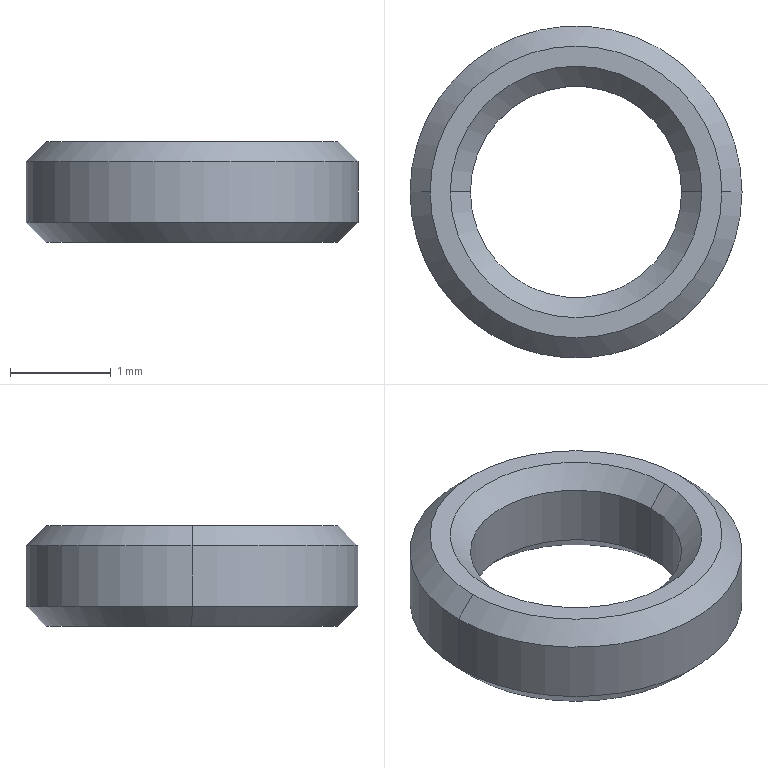Part | SolidWorks | features Chamfer 1, Extrusion 1 | 1 solid | 14 faces | box 3.3 x 3.3 x 1 mm | volume 4.411 mm3 | cone 8 | cylinder 4 | plane 2 | commonest cylinder face diameters 2.1 x2 3.3 x2
STEP:
#1=CARTESIAN_POINT('',(1.45,0.,1.));
#2=VERTEX_POINT('',#1);
#3=CARTESIAN_POINT('',(-1.45,0.,1.));
#4=VERTEX_POINT('',#3);
#5=CARTESIAN_POINT('',(0.,0.,1.));
#6=DIRECTION('',(0.,0.,1.));
#7=DIRECTION('',(1.,0.,0.));
#8=AXIS2_PLACEMENT_3D('',#5,#6,#7);
#9=CIRCLE('',#8,1.45);
#10=EDGE_CURVE('',#2,#4,#9,.T.);
#11=ORIENTED_EDGE('',*,*,#10,.F.);
#12=CARTESIAN_POINT('',(1.65,0.,0.8));
#13=VERTEX_POINT('',#12);
#14=CARTESIAN_POINT('',(1.45,0.,1.));
#15=DIRECTION('',(0.7071,0.,-0.7071));
#16=VECTOR('',#15,1000.);
#17=LINE('',#14,#16);
#18=EDGE_CURVE('',#2,#13,#17,.T.);
#19=ORIENTED_EDGE('',*,*,#18,.T.);
#20=CARTESIAN_POINT('',(-1.65,0.,0.8));
#21=VERTEX_POINT('',#20);
#22=CARTESIAN_POINT('',(0.,0.,0.8));
#23=DIRECTION('',(0.,0.,-1.));
#24=DIRECTION('',(1.,0.,0.));
#25=AXIS2_PLACEMENT_3D('',#22,#23,#24);
#26=CIRCLE('',#25,1.65);
#27=EDGE_CURVE('',#21,#13,#26,.T.);
#28=ORIENTED_EDGE('',*,*,#27,.F.);
#29=CARTESIAN_POINT('',(-1.45,0.,1.));
#30=DIRECTION('',(-0.7071,0.,-0.7071));
#31=VECTOR('',#30,1000.);
#32=LINE('',#29,#31);
#33=EDGE_CURVE('',#4,#21,#32,.T.);
#34=ORIENTED_EDGE('',*,*,#33,.F.);
#35=EDGE_LOOP('',(#11,#19,#28,#34));
#36=FACE_OUTER_BOUND('',#35,.T.);
#37=CARTESIAN_POINT('',(0.,0.,1.));
#38=DIRECTION('',(0.,0.,-1.));
#39=DIRECTION('',(-1.,0.,0.));
#40=AXIS2_PLACEMENT_3D('',#37,#38,#39);
#41=CONICAL_SURFACE('',#40,1.45,0.7854);
#42=ADVANCED_FACE('',(#36),#41,.T.);
#43=CARTESIAN_POINT('',(-1.05,0.,0.8));
#44=VERTEX_POINT('',#43);
#45=CARTESIAN_POINT('',(1.05,0.,0.8));
#46=VERTEX_POINT('',#45);
#47=CARTESIAN_POINT('',(0.,0.,0.8));
#48=DIRECTION('',(0.,0.,1.));
#49=DIRECTION('',(1.,0.,0.));
#50=AXIS2_PLACEMENT_3D('',#47,#48,#49);
#51=CIRCLE('',#50,1.05);
#52=EDGE_CURVE('',#44,#46,#51,.T.);
#53=ORIENTED_EDGE('',*,*,#52,.F.);
#54=CARTESIAN_POINT('',(-1.25,0.,1.));
#55=VERTEX_POINT('',#54);
#56=CARTESIAN_POINT('',(-1.05,0.,0.8));
#57=DIRECTION('',(-0.7071,0.,0.7071));
#58=VECTOR('',#57,1000.);
#59=LINE('',#56,#58);
#60=EDGE_CURVE('',#44,#55,#59,.T.);
#61=ORIENTED_EDGE('',*,*,#60,.T.);
#62=CARTESIAN_POINT('',(1.25,0.,1.));
#63=VERTEX_POINT('',#62);
#64=CARTESIAN_POINT('',(0.,0.,1.));
#65=DIRECTION('',(0.,0.,-1.));
#66=DIRECTION('',(1.,0.,0.));
#67=AXIS2_PLACEMENT_3D('',#64,#65,#66);
#68=CIRCLE('',#67,1.25);
#69=EDGE_CURVE('',#63,#55,#68,.T.);
#70=ORIENTED_EDGE('',*,*,#69,.F.);
#71=CARTESIAN_POINT('',(1.05,0.,0.8));
#72=DIRECTION('',(0.7071,0.,0.7071));
#73=VECTOR('',#72,1000.);
#74=LINE('',#71,#73);
#75=EDGE_CURVE('',#46,#63,#74,.T.);
#76=ORIENTED_EDGE('',*,*,#75,.F.);
#77=EDGE_LOOP('',(#53,#61,#70,#76));
#78=FACE_OUTER_BOUND('',#77,.T.);
#79=CARTESIAN_POINT('',(0.,0.,0.8));
#80=DIRECTION('',(0.,0.,1.));
#81=DIRECTION('',(1.,0.,0.));
#82=AXIS2_PLACEMENT_3D('',#79,#80,#81);
#83=CONICAL_SURFACE('',#82,1.05,0.7854);
#84=ADVANCED_FACE('',(#78),#83,.F.);
#85=CARTESIAN_POINT('',(-1.45,0.,0.));
#86=VERTEX_POINT('',#85);
#87=CARTESIAN_POINT('',(1.45,0.,0.));
#88=VERTEX_POINT('',#87);
#89=CARTESIAN_POINT('',(0.,0.,0.));
#90=DIRECTION('',(0.,0.,-1.));
#91=DIRECTION('',(1.,0.,0.));
#92=AXIS2_PLACEMENT_3D('',#89,#90,#91);
#93=CIRCLE('',#92,1.45);
#94=EDGE_CURVE('',#86,#88,#93,.T.);
#95=ORIENTED_EDGE('',*,*,#94,.F.);
#96=CARTESIAN_POINT('',(-1.65,0.,0.2));
#97=VERTEX_POINT('',#96);
#98=CARTESIAN_POINT('',(-1.65,0.,0.2));
#99=DIRECTION('',(-0.7071,0.,0.7071));
#100=VECTOR('',#99,1000.);
#101=LINE('',#98,#100);
#102=EDGE_CURVE('',#86,#97,#101,.T.);
#103=ORIENTED_EDGE('',*,*,#102,.T.);
#104=CARTESIAN_POINT('',(1.65,0.,0.2));
#105=VERTEX_POINT('',#104);
#106=CARTESIAN_POINT('',(0.,0.,0.2));
#107=DIRECTION('',(0.,0.,1.));
#108=DIRECTION('',(1.,0.,0.));
#109=AXIS2_PLACEMENT_3D('',#106,#107,#108);
#110=CIRCLE('',#109,1.65);
#111=EDGE_CURVE('',#105,#97,#110,.T.);
#112=ORIENTED_EDGE('',*,*,#111,.F.);
#113=CARTESIAN_POINT('',(1.65,0.,0.2));
#114=DIRECTION('',(0.7071,0.,0.7071));
#115=VECTOR('',#114,1000.);
#116=LINE('',#113,#115);
#117=EDGE_CURVE('',#88,#105,#116,.T.);
#118=ORIENTED_EDGE('',*,*,#117,.F.);
#119=EDGE_LOOP('',(#95,#103,#112,#118));
#120=FACE_OUTER_BOUND('',#119,.T.);
#121=CARTESIAN_POINT('',(0.,0.,0.2));
#122=DIRECTION('',(0.,0.,1.));
#123=DIRECTION('',(1.,0.,0.));
#124=AXIS2_PLACEMENT_3D('',#121,#122,#123);
#125=CONICAL_SURFACE('',#124,1.65,0.7854);
#126=ADVANCED_FACE('',(#120),#125,.T.);
#127=CARTESIAN_POINT('',(1.05,0.,0.2));
#128=VERTEX_POINT('',#127);
#129=CARTESIAN_POINT('',(-1.05,0.,0.2));
#130=VERTEX_POINT('',#129);
#131=CARTESIAN_POINT('',(0.,0.,0.2));
#132=DIRECTION('',(0.,0.,-1.));
#133=DIRECTION('',(1.,0.,0.));
#134=AXIS2_PLACEMENT_3D('',#131,#132,#133);
#135=CIRCLE('',#134,1.05);
#136=EDGE_CURVE('',#128,#130,#135,.T.);
#137=ORIENTED_EDGE('',*,*,#136,.F.);
#138=CARTESIAN_POINT('',(1.25,0.,0.));
#139=VERTEX_POINT('',#138);
#140=CARTESIAN_POINT('',(1.25,0.,0.));
#141=DIRECTION('',(0.7071,0.,-0.7071));
#142=VECTOR('',#141,1000.);
#143=LINE('',#140,#142);
#144=EDGE_CURVE('',#128,#139,#143,.T.);
#145=ORIENTED_EDGE('',*,*,#144,.T.);
#146=CARTESIAN_POINT('',(-1.25,0.,0.));
#147=VERTEX_POINT('',#146);
#148=CARTESIAN_POINT('',(0.,0.,0.));
#149=DIRECTION('',(0.,0.,1.));
#150=DIRECTION('',(1.,0.,0.));
#151=AXIS2_PLACEMENT_3D('',#148,#149,#150);
#152=CIRCLE('',#151,1.25);
#153=EDGE_CURVE('',#147,#139,#152,.T.);
#154=ORIENTED_EDGE('',*,*,#153,.F.);
#155=CARTESIAN_POINT('',(-1.25,0.,0.));
#156=DIRECTION('',(-0.7071,0.,-0.7071));
#157=VECTOR('',#156,1000.);
#158=LINE('',#155,#157);
#159=EDGE_CURVE('',#130,#147,#158,.T.);
#160=ORIENTED_EDGE('',*,*,#159,.F.);
#161=EDGE_LOOP('',(#137,#145,#154,#160));
#162=FACE_OUTER_BOUND('',#161,.T.);
#163=CARTESIAN_POINT('',(0.,0.,0.));
#164=DIRECTION('',(0.,0.,-1.));
#165=DIRECTION('',(-1.,0.,0.));
#166=AXIS2_PLACEMENT_3D('',#163,#164,#165);
#167=CONICAL_SURFACE('',#166,1.25,0.7854);
#168=ADVANCED_FACE('',(#162),#167,.F.);
#169=ORIENTED_EDGE('',*,*,#52,.T.);
#170=CARTESIAN_POINT('',(1.05,0.,1.));
#171=DIRECTION('',(0.,0.,-1.));
#172=VECTOR('',#171,1000.);
#173=LINE('',#170,#172);
#174=EDGE_CURVE('',#46,#128,#173,.T.);
#175=ORIENTED_EDGE('',*,*,#174,.T.);
#176=ORIENTED_EDGE('',*,*,#136,.T.);
#177=CARTESIAN_POINT('',(-1.05,0.,1.));
#178=DIRECTION('',(0.,0.,-1.));
#179=VECTOR('',#178,1000.);
#180=LINE('',#177,#179);
#181=EDGE_CURVE('',#44,#130,#180,.T.);
#182=ORIENTED_EDGE('',*,*,#181,.F.);
#183=EDGE_LOOP('',(#169,#175,#176,#182));
#184=FACE_OUTER_BOUND('',#183,.T.);
#185=CARTESIAN_POINT('',(0.,0.,1.));
#186=DIRECTION('',(0.,0.,-1.));
#187=DIRECTION('',(-1.,0.,0.));
#188=AXIS2_PLACEMENT_3D('',#185,#186,#187);
#189=CYLINDRICAL_SURFACE('',#188,1.05);
#190=ADVANCED_FACE('',(#184),#189,.F.);
#191=ORIENTED_EDGE('',*,*,#27,.T.);
#192=CARTESIAN_POINT('',(1.65,0.,1.));
#193=DIRECTION('',(0.,0.,-1.));
#194=VECTOR('',#193,1000.);
#195=LINE('',#192,#194);
#196=EDGE_CURVE('',#13,#105,#195,.T.);
#197=ORIENTED_EDGE('',*,*,#196,.T.);
#198=ORIENTED_EDGE('',*,*,#111,.T.);
#199=CARTESIAN_POINT('',(-1.65,0.,1.));
#200=DIRECTION('',(0.,0.,-1.));
#201=VECTOR('',#200,1000.);
#202=LINE('',#199,#201);
#203=EDGE_CURVE('',#21,#97,#202,.T.);
#204=ORIENTED_EDGE('',*,*,#203,.F.);
#205=EDGE_LOOP('',(#191,#197,#198,#204));
#206=FACE_OUTER_BOUND('',#205,.T.);
#207=CARTESIAN_POINT('',(0.,0.,1.));
#208=DIRECTION('',(0.,0.,-1.));
#209=DIRECTION('',(-1.,0.,0.));
#210=AXIS2_PLACEMENT_3D('',#207,#208,#209);
#211=CYLINDRICAL_SURFACE('',#210,1.65);
#212=ADVANCED_FACE('',(#206),#211,.T.);
#213=ORIENTED_EDGE('',*,*,#69,.T.);
#214=CARTESIAN_POINT('',(0.,0.,1.));
#215=DIRECTION('',(0.,0.,-1.));
#216=DIRECTION('',(1.,0.,0.));
#217=AXIS2_PLACEMENT_3D('',#214,#215,#216);
#218=CIRCLE('',#217,1.25);
#219=EDGE_CURVE('',#55,#63,#218,.T.);
#220=ORIENTED_EDGE('',*,*,#219,.T.);
#221=EDGE_LOOP('',(#213,#220));
#222=FACE_BOUND('',#221,.T.);
#223=CARTESIAN_POINT('',(0.,0.,1.));
#224=DIRECTION('',(0.,0.,1.));
#225=DIRECTION('',(1.,0.,0.));
#226=AXIS2_PLACEMENT_3D('',#223,#224,#225);
#227=CIRCLE('',#226,1.45);
#228=EDGE_CURVE('',#4,#2,#227,.T.);
#229=ORIENTED_EDGE('',*,*,#228,.T.);
#230=ORIENTED_EDGE('',*,*,#10,.T.);
#231=EDGE_LOOP('',(#229,#230));
#232=FACE_OUTER_BOUND('',#231,.T.);
#233=CARTESIAN_POINT('',(0.,0.,1.));
#234=DIRECTION('',(0.,0.,1.));
#235=DIRECTION('',(1.,0.,0.));
#236=AXIS2_PLACEMENT_3D('',#233,#234,#235);
#237=PLANE('',#236);
#238=ADVANCED_FACE('',(#222,#232),#237,.T.);
#239=ORIENTED_EDGE('',*,*,#153,.T.);
#240=CARTESIAN_POINT('',(0.,0.,0.));
#241=DIRECTION('',(0.,0.,1.));
#242=DIRECTION('',(1.,0.,0.));
#243=AXIS2_PLACEMENT_3D('',#240,#241,#242);
#244=CIRCLE('',#243,1.25);
#245=EDGE_CURVE('',#139,#147,#244,.T.);
#246=ORIENTED_EDGE('',*,*,#245,.T.);
#247=EDGE_LOOP('',(#239,#246));
#248=FACE_BOUND('',#247,.T.);
#249=CARTESIAN_POINT('',(0.,0.,0.));
#250=DIRECTION('',(0.,0.,-1.));
#251=DIRECTION('',(1.,0.,0.));
#252=AXIS2_PLACEMENT_3D('',#249,#250,#251);
#253=CIRCLE('',#252,1.45);
#254=EDGE_CURVE('',#88,#86,#253,.T.);
#255=ORIENTED_EDGE('',*,*,#254,.T.);
#256=ORIENTED_EDGE('',*,*,#94,.T.);
#257=EDGE_LOOP('',(#255,#256));
#258=FACE_OUTER_BOUND('',#257,.T.);
#259=CARTESIAN_POINT('',(0.,0.,0.));
#260=DIRECTION('',(0.,0.,1.));
#261=DIRECTION('',(1.,0.,0.));
#262=AXIS2_PLACEMENT_3D('',#259,#260,#261);
#263=PLANE('',#262);
#264=ADVANCED_FACE('',(#248,#258),#263,.F.);
#265=ORIENTED_EDGE('',*,*,#196,.F.);
#266=CARTESIAN_POINT('',(0.,0.,0.8));
#267=DIRECTION('',(0.,0.,-1.));
#268=DIRECTION('',(1.,0.,0.));
#269=AXIS2_PLACEMENT_3D('',#266,#267,#268);
#270=CIRCLE('',#269,1.65);
#271=EDGE_CURVE('',#13,#21,#270,.T.);
#272=ORIENTED_EDGE('',*,*,#271,.T.);
#273=ORIENTED_EDGE('',*,*,#203,.T.);
#274=CARTESIAN_POINT('',(0.,0.,0.2));
#275=DIRECTION('',(0.,0.,1.));
#276=DIRECTION('',(1.,0.,0.));
#277=AXIS2_PLACEMENT_3D('',#274,#275,#276);
#278=CIRCLE('',#277,1.65);
#279=EDGE_CURVE('',#97,#105,#278,.T.);
#280=ORIENTED_EDGE('',*,*,#279,.T.);
#281=EDGE_LOOP('',(#265,#272,#273,#280));
#282=FACE_OUTER_BOUND('',#281,.T.);
#283=CARTESIAN_POINT('',(0.,0.,1.));
#284=DIRECTION('',(0.,0.,-1.));
#285=DIRECTION('',(-1.,0.,0.));
#286=AXIS2_PLACEMENT_3D('',#283,#284,#285);
#287=CYLINDRICAL_SURFACE('',#286,1.65);
#288=ADVANCED_FACE('',(#282),#287,.T.);
#289=ORIENTED_EDGE('',*,*,#174,.F.);
#290=CARTESIAN_POINT('',(0.,0.,0.8));
#291=DIRECTION('',(0.,0.,1.));
#292=DIRECTION('',(1.,0.,0.));
#293=AXIS2_PLACEMENT_3D('',#290,#291,#292);
#294=CIRCLE('',#293,1.05);
#295=EDGE_CURVE('',#46,#44,#294,.T.);
#296=ORIENTED_EDGE('',*,*,#295,.T.);
#297=ORIENTED_EDGE('',*,*,#181,.T.);
#298=CARTESIAN_POINT('',(0.,0.,0.2));
#299=DIRECTION('',(0.,0.,-1.));
#300=DIRECTION('',(1.,0.,0.));
#301=AXIS2_PLACEMENT_3D('',#298,#299,#300);
#302=CIRCLE('',#301,1.05);
#303=EDGE_CURVE('',#130,#128,#302,.T.);
#304=ORIENTED_EDGE('',*,*,#303,.T.);
#305=EDGE_LOOP('',(#289,#296,#297,#304));
#306=FACE_OUTER_BOUND('',#305,.T.);
#307=CARTESIAN_POINT('',(0.,0.,1.));
#308=DIRECTION('',(0.,0.,-1.));
#309=DIRECTION('',(-1.,0.,0.));
#310=AXIS2_PLACEMENT_3D('',#307,#308,#309);
#311=CYLINDRICAL_SURFACE('',#310,1.05);
#312=ADVANCED_FACE('',(#306),#311,.F.);
#313=ORIENTED_EDGE('',*,*,#144,.F.);
#314=ORIENTED_EDGE('',*,*,#303,.F.);
#315=ORIENTED_EDGE('',*,*,#159,.T.);
#316=ORIENTED_EDGE('',*,*,#245,.F.);
#317=EDGE_LOOP('',(#313,#314,#315,#316));
#318=FACE_OUTER_BOUND('',#317,.T.);
#319=CARTESIAN_POINT('',(0.,0.,0.));
#320=DIRECTION('',(0.,0.,-1.));
#321=DIRECTION('',(-1.,0.,0.));
#322=AXIS2_PLACEMENT_3D('',#319,#320,#321);
#323=CONICAL_SURFACE('',#322,1.25,0.7854);
#324=ADVANCED_FACE('',(#318),#323,.F.);
#325=ORIENTED_EDGE('',*,*,#102,.F.);
#326=ORIENTED_EDGE('',*,*,#254,.F.);
#327=ORIENTED_EDGE('',*,*,#117,.T.);
#328=ORIENTED_EDGE('',*,*,#279,.F.);
#329=EDGE_LOOP('',(#325,#326,#327,#328));
#330=FACE_OUTER_BOUND('',#329,.T.);
#331=CARTESIAN_POINT('',(0.,0.,0.2));
#332=DIRECTION('',(0.,0.,1.));
#333=DIRECTION('',(1.,0.,0.));
#334=AXIS2_PLACEMENT_3D('',#331,#332,#333);
#335=CONICAL_SURFACE('',#334,1.65,0.7854);
#336=ADVANCED_FACE('',(#330),#335,.T.);
#337=ORIENTED_EDGE('',*,*,#60,.F.);
#338=ORIENTED_EDGE('',*,*,#295,.F.);
#339=ORIENTED_EDGE('',*,*,#75,.T.);
#340=ORIENTED_EDGE('',*,*,#219,.F.);
#341=EDGE_LOOP('',(#337,#338,#339,#340));
#342=FACE_OUTER_BOUND('',#341,.T.);
#343=CARTESIAN_POINT('',(0.,0.,0.8));
#344=DIRECTION('',(0.,0.,1.));
#345=DIRECTION('',(1.,0.,0.));
#346=AXIS2_PLACEMENT_3D('',#343,#344,#345);
#347=CONICAL_SURFACE('',#346,1.05,0.7854);
#348=ADVANCED_FACE('',(#342),#347,.F.);
#349=ORIENTED_EDGE('',*,*,#18,.F.);
#350=ORIENTED_EDGE('',*,*,#228,.F.);
#351=ORIENTED_EDGE('',*,*,#33,.T.);
#352=ORIENTED_EDGE('',*,*,#271,.F.);
#353=EDGE_LOOP('',(#349,#350,#351,#352));
#354=FACE_OUTER_BOUND('',#353,.T.);
#355=CARTESIAN_POINT('',(0.,0.,1.));
#356=DIRECTION('',(0.,0.,-1.));
#357=DIRECTION('',(-1.,0.,0.));
#358=AXIS2_PLACEMENT_3D('',#355,#356,#357);
#359=CONICAL_SURFACE('',#358,1.45,0.7854);
#360=ADVANCED_FACE('',(#354),#359,.T.);
#361=CLOSED_SHELL('',(#42,#84,#126,#168,#190,#212,#238,#264,#288,#312,#324,#336,#348,#360));
#362=MANIFOLD_SOLID_BREP('',#361);
#363=CARTESIAN_POINT('',(0.,0.,0.));
#364=DIRECTION('',(0.,0.,1.));
#365=DIRECTION('',(1.,0.,0.));
#366=AXIS2_PLACEMENT_3D('',#363,#364,#365);
#367=(LENGTH_UNIT()NAMED_UNIT(*)SI_UNIT(.MILLI.,.METRE.));
#368=UNCERTAINTY_MEASURE_WITH_UNIT(LENGTH_MEASURE(0.00001),#367,'','');
#369=(NAMED_UNIT(*)PLANE_ANGLE_UNIT()SI_UNIT($,.RADIAN.));
#370=(NAMED_UNIT(*)SI_UNIT($,.STERADIAN.)SOLID_ANGLE_UNIT());
#371=(GEOMETRIC_REPRESENTATION_CONTEXT(3)GLOBAL_UNCERTAINTY_ASSIGNED_CONTEXT((#368))GLOBAL_UNIT_ASSIGNED_CONTEXT((#367,#369,#370))REPRESENTATION_CONTEXT('',''));
#372=ADVANCED_BREP_SHAPE_REPRESENTATION('',(#362,#366),#371);